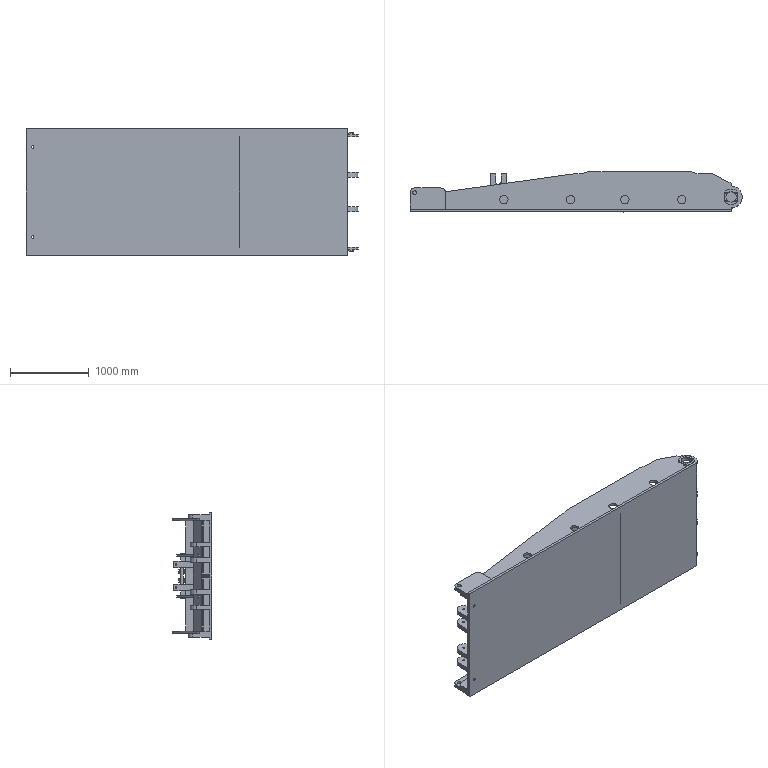Part | NX | features 顶梁 2 | 1 solid | 429 faces | box 4215 x 507.464 x 1600 mm | volume 647411376 mm3 | plane 336 | cylinder 87 | spline 4 | sphere 2 | commonest cylinder face diameters 107 x14 160 x8 30 x6 40 x6 158.292 x5 20 x4